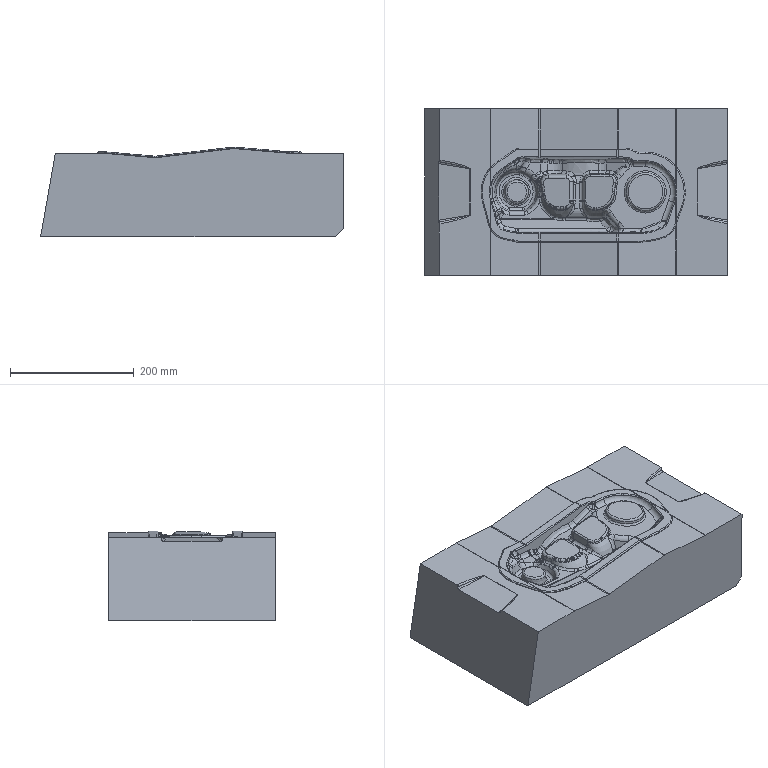NC program | NX | posted with a generic post | part box 490.523 x 270 x 145.452 mm
Lines 1 to 892 of 192747:
N10 G17 G21 G94 G90
(FIXED_CONTOUR , TOOL : 6.)
N12 T00 M6
N14 G54
N16 G17 G0 G90 X-85.619 Y71.107 S3000 M3
N18 G43 Z100. H0
N20 Z5.2
N22 G94 G1 Z0.4 F2500.
N24 X-86.787 Y69.405
N26 X-87.928 Y67.935
N28 Y67.84
N30 X-85.569 Y70.881 Z0.2
N32 Y71.005
N34 X-84.81 Y72.233
N36 X-84.104 Y73.498
N38 X-82.98 Y75.839
N40 X-82.866 Y76.096 Z0.178
N42 X-82.621 Y76.604 Z0.133
N44 X-82.287 Y77.38 Z0.067
N46 X-81.952 Y78.155 Z0.
N48 X-81.954 Y78.15
N50 X-83.083 Y75.364
N52 Y75.2
N54 Z5.2
N56 G0 Z100.
N58 X-19.722 Y93.035
N60 Z1.6
N62 G1 Z-3.456
N64 X-13.17 Y91.559
N66 X-6.598 Y90.205
N68 X-0.002 Y88.972
N70 X-0.001 Y89.016 Z-3.549
N72 X0. Y89.051 Z-3.642
N74 G2 X-18.281 Y92.786 R370.357
N76 G1 Y92.803
N78 Y92.807
N80 X-16.767 Y92.538 Z-3.828
N82 Y92.534
N84 Y92.517
N86 X-15.395 Y92.209
N88 X-7.747 Y90.592
N90 X0. Y89.128
N92 Y89.17 Z-3.921
N94 Y89.198 Z-4.014
N96 X-6.896 Y90.494
N98 X-13.7 Y91.909
N100 X-15.252 Y92.251
N102 Y92.271
N104 X-14.495 Y92.137 Z-4.107
N106 X-14.174 Y92.092 Z-4.138
N108 X-13.99 Y92.047 Z-4.169
N110 X-13.737 Y92.003 Z-4.2
N112 Y91.998
N114 Y91.981
N116 X-12.039 Y91.614
N118 X-6.063 Y90.392
N120 X0. Y89.263
N122 Y89.295 Z-4.293
N124 Y89.316 Z-4.386
N126 X-2.373 Y89.761
N128 X-10.421 Y91.327
N130 X-12.223 Y91.711
N132 Y91.729
N134 Y91.733
N136 X-10.708 Y91.465 Z-4.571
N138 Y91.461
N140 Y91.444
N142 X-8.497 Y90.986
N144 X0. Y89.367
N146 Y89.396 Z-4.664
N148 Y89.412 Z-4.757
N150 X-6.435 Y90.62
N152 X-9.194 Y91.175
N154 Y91.192
N156 Y91.197
N158 X-7.679 Y90.929 Z-4.943
N160 Y90.908
N162 X-4.099 Y90.207
N164 X0. Y89.447
N166 Y89.467 Z-5.036
N168 Y89.477 Z-5.129
N170 X-0.578 Y89.582
N172 X-6.164 Y90.641
N174 Y90.657
N176 Y90.662
N178 X-4.65 Y90.391 Z-5.315
N180 Y90.387
N182 Y90.369
N184 X-0.004 Y89.506
N186 X-0.003 Y89.526 Z-5.501
N188 X-3.135 Y90.103
N190 Y90.12
N192 Y90.124
N194 Z1.6
N196 G0 Z100.
N198 X0.004 Y180.967
N200 Z1.6
N202 G1 Z-3.614
N204 X-8.082 Y179.426
N206 X-16.134 Y177.736
N208 X-18.504 Y177.176
N210 Y177.159
N212 X-16.962 Y177.432 Z-3.804
N214 Y177.449
N216 X-14.338 Y178.042
N218 X-7.468 Y179.472
N220 X-0.573 Y180.773
N222 X0.003 Y180.888
N224 X0.004 Y180.841 Z-3.898
N226 Y180.822 Z-3.993
N228 X-3.565 Y180.152
N230 X-4.164 Y180.056
N232 X-12.543 Y178.358
N234 X-15.42 Y177.72
N236 Y177.704
N238 X-13.878 Y177.978 Z-4.182
N240 Y177.995
N242 X-12.26 Y178.347
N244 X-7.322 Y179.366
N246 X-2.368 Y180.307
N248 X0.004 Y180.748
N250 Y180.71 Z-4.277
N252 Y180.69 Z-4.372
N254 X-8.353 Y179.115
N256 X-12.336 Y178.268
N258 Y178.251
N260 X-10.794 Y178.524 Z-4.561
N262 Y178.541
N264 X-8.56 Y179.001
N266 X0.004 Y180.638
N268 Y180.608 Z-4.656
N270 Y180.591 Z-4.75
N272 X-6.576 Y179.352
N274 X-9.252 Y178.814
N276 Y178.797
N278 X-7.71 Y179.068 Z-4.94
N280 Y179.085
N282 X-6.558 Y179.318
N284 X0.003 Y180.565
N286 X0. Y180.534 Z-5.034
N288 Y180.528 Z-5.129
N290 X-0.573 Y180.43
N292 X-6.168 Y179.358
N294 Y179.341
N296 X-4.626 Y179.617 Z-5.318
N298 Y179.634
N300 X0.003 Y180.501
N302 Y180.475 Z-5.508
N304 X-3.084 Y179.905
N306 Y179.888
N308 Z1.6
N310 G0 Z100.
N312 X-164.272 Y125.065
N314 Z11.2
N316 G1 Z5.572
N318 G2 X-164.29 Y145.109 R32.234
N320 G1 X-163.918 Y146.241 Z5.539
N322 X-163.819 Y146.523 Z5.531
N324 X-163.28 Y147.922 Z5.489
N326 X-162.67 Y149.293 Z5.448
N328 X-162.405 Y149.83 Z5.431
N330 X-161.863 Y150.895 Z5.398
N332 X-161.42 Y151.668 Z5.373
N334 G3 X-161.471 Y118.63 R32.426
N336 G1 X-161.317 Y118.389 Z5.362
N338 X-161.034 Y117.89 Z5.34
N340 X-160.268 Y116.677 Z5.285
N342 X-160.109 Y116.438 Z5.274
N344 X-159.278 Y115.268 Z5.219
N346 X-158.752 Y114.592 Z5.186
N348 X-158.573 Y114.37 Z5.175
N350 X-158.734 Y114.56
N352 X-159.247 Y115.191
N354 X-159.867 Y116.038
N356 G2 X-165.436 Y141.376 R32.467
N358 X-158.607 Y155.835 R32.151
N360 G1 X-158.278 Y156.266 Z5.131
N362 X-157.935 Y156.685 Z5.087
N364 X-157.237 Y157.513 Z4.998
N366 X-157.05 Y157.708 Z4.976
N368 G3 X-165.983 Y138.11 R32.384
N370 G1 X-166.115 Y135.573
N372 X-166.05 Y133.033
N374 X-165.965 Y131.842
N376 X-165.88 Y131.246
N378 X-165.832 Y130.764
N380 X-165.731 Y130.054
N382 X-165.615 Y129.458
N384 X-165.524 Y128.862
N386 G3 X-157.059 Y112.536 R32.534
N388 G1 X-156.677 Y112.126 Z4.948
N390 X-156.098 Y111.515 Z4.906
N392 X-155.489 Y110.933 Z4.863
N394 X-154.877 Y110.356 Z4.82
N396 X-154.243 Y109.808 Z4.778
N398 G2 X-165.831 Y130.354 R32.559
N400 X-165.365 Y142.358 R32.535
N402 X-160.052 Y154.259 R32.552
N404 G1 X-158.428 Y156.335
N406 X-156.639 Y158.271
N408 X-155.462 Y159.386
N410 X-154.231 Y160.442
N412 X-153.779 Y160.824 Z4.745
N414 X-153.553 Y161.016 Z4.728
N416 X-152.384 Y161.924 Z4.646
N418 X-151.419 Y162.605 Z4.579
N420 X-152.824 Y161.638
N422 X-153.259 Y161.294
N424 X-153.616 Y161.042
N426 G3 X-165.08 Y143.76 R32.349
N428 G1 X-165.698 Y141.015
N430 X-166.086 Y138.227
N432 X-166.241 Y135.417
N434 G3 X-159.781 Y115.485 R33.243
N436 G1 X-158.044 Y113.343
N438 X-156.13 Y111.357
N440 X-154.054 Y109.541
N442 X-153.616 Y109.196
N444 X-153.259 Y108.944
N446 X-152.661 Y108.48
N448 X-151.408 Y107.622
N450 X-151.177 Y107.471 Z4.563
N452 X-150.951 Y107.312 Z4.546
N454 X-149.551 Y106.429 Z4.447
N456 X-148.831 Y106.025 Z4.397
N458 X-148.594 Y105.885 Z4.381
N460 G2 X-164.177 Y123.473 R32.567
N462 X-157.009 Y158.119 R33.181
N464 X-148.592 Y164.345 R32.559
N466 G1 X-148.09 Y164.623 Z4.345
N468 X-146.805 Y165.267 Z4.255
N470 X-146.282 Y165.503 Z4.219
N472 X-145.756 Y165.731 Z4.182
N474 G3 X-163.495 Y148.58 R32.442
N476 X-165.617 Y128.266 R33.346
N478 G1 X-165.352 Y127.074
N480 X-165.202 Y126.478
N482 G3 X-153.858 Y109.164 R33.176
N484 G1 X-153.259 Y108.733
N486 X-152.661 Y108.268
N488 X-152.289 Y108.004
N490 G3 X-145.766 Y104.506 R33.729
N492 G1 X-145.51 Y104.404 Z4.164
N494 X-145.258 Y104.291 Z4.146
N496 X-144.489 Y103.987 Z4.092
N498 X-143.715 Y103.695 Z4.038
N500 X-142.93 Y103.442 Z3.984
N502 G2 X-151.418 Y107.34 R31.827
N504 X-160.993 Y116.943 R32.498
N506 X-155.055 Y160.163 R33.378
N508 X-142.948 Y166.794 R32.328
N510 G1 X-142.666 Y166.881 Z3.964
N512 X-142.106 Y167.07 Z3.924
N514 X-140.682 Y167.456 Z3.825
N516 X-140.396 Y167.526 Z3.805
N518 X-140.108 Y167.586 Z3.785
N520 G3 X-155.265 Y160.021 R31.836
N522 X-163.084 Y149.667 R33.015
N524 X-157.427 Y112.312 R33.489
N526 G1 X-155.449 Y110.37
N528 X-153.315 Y108.6
N530 G3 X-140.119 Y102.657 R31.84
N532 G1 X-138.996 Y102.402 Z3.706
N534 X-137.578 Y102.166 Z3.607
N536 X-137.294 Y102.126 Z3.587
N538 X-139.945 Y102.528
N540 G2 X-158.648 Y113.628 R32.465
N542 G1 X-160.302 Y115.768
N544 X-161.774 Y118.038
N546 X-163.053 Y120.422
N548 G2 X-166.231 Y131.321 R33.907
N550 X-153.796 Y161.324 R33.477
N552 X-137.314 Y168.103 R31.937
N554 G1 X-137.032 Y168.151 Z3.567
N556 X-135.9 Y168.288 Z3.488
N558 X-135.616 Y168.316 Z3.468
N560 X-134.481 Y168.387 Z3.388
N562 G3 X-150.082 Y163.93 R31.865
N564 G1 X-152.328 Y162.479
N566 X-154.457 Y160.861
N568 G3 X-164.036 Y122.558 R33.577
N570 X-152.985 Y108.227 R33.222
N572 X-134.481 Y101.859 R32.008
N574 G1 X-134.201 Y101.828 Z3.369
N576 X-133.921 Y101.812 Z3.349
N578 X-132.52 Y101.791 Z3.25
N580 X-131.682 Y101.814 Z3.19
N582 G2 X-149.667 Y106.013 R32.181
N584 X-164.956 Y125.02 R33.356
N586 X-153.743 Y161.482 R33.609
N588 X-137.125 Y168.306 R32.658
N590 G1 X-134.405 Y168.481
N592 X-131.683 Y168.425
N594 X-130.838 Y168.406 Z3.13
N596 X-129.155 Y168.261 Z3.011
N598 X-128.877 Y168.22 Z2.991
N600 X-131.57 Y168.509
N602 G3 X-137.692 Y168.311 R35.795
N604 X-152.062 Y162.767 R32.727
N606 G1 X-154.457 Y160.954
N608 G3 X-159.986 Y115.156 R33.662
N610 G1 X-158.363 Y113.137
N612 G3 X-147.904 Y105.025 R33.306
N614 X-128.879 Y102.017 R32.12
N616 G1 X-128.308 Y102.08 Z2.952
N618 X-127.737 Y102.153 Z2.912
N620 X-127.453 Y102.198 Z2.892
N622 X-126.325 Y102.409 Z2.813
N624 X-126.046 Y102.472 Z2.793
N626 G2 X-148.003 Y105.025 R32.317
N628 G1 X-150.392 Y106.346
N630 G2 X-160.327 Y115.576 R33.664
N632 X-144.147 Y166.838 R33.645
N634 X-126.058 Y167.769 R32.242
N636 G1 X-125.775 Y167.73 Z2.773
N638 X-124.665 Y167.471 Z2.694
N640 X-124.388 Y167.404 Z2.674
N642 X-123.295 Y167.09 Z2.595
N644 G3 X-139.592 Y168.118 R32.546
N646 G1 X-142.053 Y167.537
N648 X-144.462 Y166.768
N650 X-146.805 Y165.817
N652 X-149.068 Y164.689
N654 X-151.488 Y163.233
N656 X-153.778 Y161.58
N658 X-155.921 Y159.74
N660 G3 X-157.017 Y111.58 R33.682
N662 G1 X-156.852 Y111.407
N664 G3 X-139.237 Y102.045 R33.451
N666 X-124.723 Y102.716 R32.48
N668 G1 X-123.284 Y103.155
N670 X-122.997 Y103.225 Z2.575
N672 X-122.713 Y103.308 Z2.555
N674 X-121.317 Y103.788 Z2.456
N676 X-120.493 Y104.108 Z2.396
N678 X-120.928 Y103.931
N680 X-121.118 Y103.833
N682 X-121.527 Y103.692
N684 X-122.697 Y103.237
N686 G2 X-129.31 Y101.709 R37.844
N688 X-134.1 Y101.457 R37.107
N690 G1 X-134.699 Y101.499
N692 G2 X-145.525 Y103.833 R32.829
N694 G1 X-146.075 Y104.08
N696 X-146.673 Y104.329
N698 G2 X-151.438 Y163.304 R33.725
N700 X-139.114 Y168.256 R33.424
N702 X-120.49 Y166.129 R32.461
N704 G1 X-119.714 Y165.829 Z2.342
N706 X-118.202 Y165.138 Z2.234
N708 X-117.711 Y164.883 Z2.198
N710 G3 X-143.895 Y167.038 R32.59
N712 X-155.146 Y160.521 R33.727
N714 G1 X-157.129 Y158.641
N716 X-158.953 Y156.607
N718 X-160.607 Y154.432
N720 X-162.079 Y152.13
N722 G3 X-150.864 Y106.538 R33.734
N724 X-131.312 Y101.464 R33.198
N726 X-117.728 Y105.347 R32.66
N728 G1 X-116.949 Y105.737 Z2.143
N730 X-116.694 Y105.875 Z2.125
N732 X-115.44 Y106.602 Z2.035
N734 X-114.954 Y106.915 Z1.999
N736 G2 X-137.826 Y101.705 R32.613
N738 G1 X-140.427 Y102.184
N740 X-142.983 Y102.868
N742 X-145.476 Y103.752
N744 X-146.075 Y104.022
N746 X-146.673 Y104.262
N748 X-147.045 Y104.429
N750 X-148.469 Y105.127
N752 X-149.068 Y105.448
N754 X-151.464 Y106.881
N756 G2 X-161.247 Y116.7 R33.77
N758 X-147.284 Y165.693 R33.771
N760 X-124.949 Y167.824 R32.947
N762 X-114.962 Y163.331 R32.648
N764 G1 X-114.009 Y162.723 Z1.933
N766 X-112.634 Y161.73 Z1.834
N768 X-112.192 Y161.381 Z1.801
N770 G3 X-136.93 Y168.684 R32.74
N772 X-150.266 Y164.136 R33.753
N774 X-153.137 Y108.024 R33.776
N776 X-131.385 Y101.369 R33.627
N778 G1 X-128.772 Y101.605
N780 G3 X-112.189 Y108.864 R32.871
N782 G1 X-111.518 Y109.387 Z1.755
N784 X-111.088 Y109.756 Z1.724
N786 X-110.237 Y110.505 Z1.663
N788 X-109.421 Y111.287 Z1.602
N790 G2 X-128.439 Y101.606 R33.041
N792 X-145.782 Y103.833 R33.43
N794 X-153.441 Y162.018 R33.798
N796 G1 X-151.108 Y163.642
N798 X-148.646 Y165.064
N800 X-146.075 Y166.274
N802 X-145.782 Y166.405
N804 G2 X-123.666 Y167.597 R33.229
N806 X-109.419 Y158.947 R33.26
N808 G1 X-108.997 Y158.535 Z1.583
N810 X-107.994 Y157.448 Z1.536
N812 X-107.229 Y156.542 Z1.498
N814 X-106.851 Y156.086 Z1.479
N816 X-105.956 Y154.91 Z1.432
N818 X-105.785 Y154.67 Z1.422
N820 X-105.623 Y154.424 Z1.413
N822 X-105.455 Y154.183 Z1.404
N824 G3 X-113.728 Y162.77 R32.793
N826 G1 X-116.018 Y164.278
N828 X-118.423 Y165.595
N830 X-120.928 Y166.711
N832 G3 X-146.075 Y166.303 R33.323
N834 G1 X-148.568 Y165.137
N836 X-150.959 Y163.773
N838 X-153.23 Y162.218
N840 X-155.368 Y160.483
N842 G3 X-157.139 Y111.44 R33.804
N844 X-128.431 Y101.575 R33.872
N846 X-105.482 Y116.019 R32.97
N848 G1 X-105.148 Y116.489 Z1.383
N850 X-104.985 Y116.726 Z1.372
N852 X-104.219 Y117.949 Z1.32
N854 X-104.07 Y118.196 Z1.31
N856 X-103.505 Y119.203 Z1.268
N858 X-103.236 Y119.712 Z1.247
N860 X-102.724 Y120.74 Z1.205
N862 G2 X-121.341 Y103.328 R33.391
N864 G1 X-123.922 Y102.477
N866 G2 X-153.244 Y108.004 R33.808
N868 G1 X-155.438 Y109.786
N870 X-157.476 Y111.744
N872 X-159.343 Y113.866
N874 G2 X-153.816 Y161.789 R33.799
N876 G1 X-153.244 Y162.234
N878 G2 X-126.317 Y168.342 R33.905
N880 X-103.898 Y151.813 R33.206
N882 G1 X-102.783 Y149.621
N884 X-102.706 Y149.454
N886 Z6.605
N888 G0 Z9.005
N890 X-99.98 Y140.994
N892 Z6.605
N894 G1 Z1.007
N896 G3 X-110.734 Y160.55 R34.127
N898 X-133.196 Y169.017 R33.186
N900 X-166.844 Y136.897 R33.962
N902 X-146.727 Y104.155 R33.873
N904 X-125.119 Y102.136 R33.922
N906 G1 X-123.922 Y102.441
N908 G3 X-103.56 Y118.837 R33.366
N910 X-99.963 Y129.342 R34.667
N912 G1 Z6.4
N914 G0 Z100.
N916 X-102.441 Y149.336
N918 Z6.4
N920 G1 Z0.808
N922 G2 X-107.461 Y112.96 R34.453
N924 X-118.524 Y104.429 R33.412
N926 X-147.871 Y104.668 R33.813
N928 X-164.557 Y147.558 R33.857
N930 X-121.377 Y167.003 R34.003
N932 X-104.949 Y153.891 R33.172
N934 G1 X-103.605 Y151.663
N936 X-102.441 Y149.336
N938 X-102.394 Y149.357 Z0.709
N940 X-102.377 Y149.365 Z0.61
N942 G3 X-111.814 Y161.615 R33.797
N944 X-123.628 Y167.76 R33.153
N946 X-165.845 Y143.76 R34.05
N948 X-149.068 Y105.245 R33.907
N950 X-121.875 Y103.028 R34.083
N952 X-108.459 Y111.762 R32.992
N954 X-99.872 Y128.835 R34.
N956 X-101.461 Y147.154 R34.535
N958 G1 X-102.377 Y149.365
N960 Z6.4
N962 G0 Z100.
N964 X-167.07 Y137.895
N966 Z10.
N968 G1 Z0.411
N970 Y136.445
N972 X-166.998 Y137.308
N974 X-166.638 Y140.185
N976 G2 X-128.546 Y168.789 R34.085
N978 X-102.761 Y150.315 R33.363
N980 X-109.732 Y110.388 R34.322
N982 X-129.31 Y101.366 R33.362
N984 G1 X-129.909 Y101.292
N986 X-131.106 Y101.205
N988 X-132.226 Y101.181
N990 G2 X-166.83 Y131.573 R34.059
N992 G1 X-167.028 Y133.406
N994 Z9.561
N996 G0 Z11.961
N998 X-164.662 Y122.521
N1000 Z9.561
N1002 G1 Z0.213
N1004 X-164.635 Y122.476
N1006 X-164.036 Y121.15
N1008 G3 X-118.418 Y104.394 R34.154
N1010 X-104.571 Y116.591 R33.416
N1012 X-107.756 Y157.869 R34.349
N1014 X-123.632 Y167.808 R33.802
N1016 X-164.542 Y147.932 R34.195
N1018 G1 X-164.658 Y147.769
N1020 Z9.363
N1022 G0 Z11.763
N1024 X-162.355 Y152.492
N1026 Z9.363
N1028 G1 Z0.014
N1030 X-161.641 Y153.524
N1032 G2 X-114.564 Y163.724 R34.161
N1034 X-100.352 Y144.37 R33.674
N1036 X-106.376 Y113.963 R34.352
N1038 X-130.508 Y101.213 R33.711
N1040 X-161.788 Y116.943 R34.169
N1042 G1 X-162.361 Y117.747
N1044 Z9.164
N1046 G0 Z11.564
N1048 X-160.026 Y114.272
N1050 Z9.164
N1052 G1 Z-0.184
N1054 X-159.712 Y113.964
N1056 G3 X-128.584 Y101.398 R34.232
N1058 X-100.765 Y124.341 R33.707
N1060 G1 X-100.455 Y125.286
N1062 X-100.295 Y125.882
N1064 G3 X-106.559 Y156.571 R34.301
N1066 X-118.597 Y165.965 R34.067
N1068 X-158.18 Y158.062 R34.283
N1070 G1 X-159.965 Y156.014
N1072 X-160.019 Y155.972
N1074 Z8.966
N1076 G0 Z11.366
N1078 X-157.686 Y158.716
N1080 Z8.966
N1082 G1 Z-0.383
N1084 X-157.403 Y158.929
N1086 G2 X-113.172 Y162.83 R34.263
N1088 X-110.151 Y160.404 R36.808
N1090 X-99.547 Y141.376 R34.02
N1092 G1 X-99.463 Y140.78
N1094 X-99.374 Y140.353
N1096 G2 X-101.276 Y122.776 R34.557
N1098 X-112.227 Y108.116 R33.746
N1100 X-132.304 Y101.1 R33.979
N1102 X-156.45 Y110.388 R34.253
N1104 G1 X-157.599 Y111.468
N1106 X-157.682 Y111.518
N1108 Z8.767
N1110 G0 Z11.167
N1112 X-155.345 Y109.27
N1114 Z8.767
N1116 G1 Z-0.581
N1118 X-155.195 Y109.196
N1120 X-154.444 Y108.6
N1122 G3 X-110.151 Y109.807 R34.285
N1124 X-110.151 Y160.431 R34.166
N1126 X-152.862 Y162.83 R34.281
N1128 G1 X-153.259 Y162.55
N1130 X-155.303 Y160.993
N1132 Z8.569
N1134 G0 Z10.969
N1136 X-153.016 Y162.841
N1138 Z8.569
N1140 G1 Z-0.78
N1142 X-152.661 Y163.02
N1144 G2 X-108.763 Y159.131 R34.334
N1146 X-108.648 Y111.224 R34.171
N1148 X-152.661 Y107.219 R34.331
N1150 G1 X-153.002 Y107.392
N1152 Z8.37
N1154 G0 Z10.77
N1156 X-150.644 Y105.816
N1158 Z8.37
N1160 G1 Z-0.978
N1162 X-150.492 Y105.783
N1164 X-149.154 Y105.069
N1166 G3 X-106.559 Y113.542 R34.248
N1168 X-102.545 Y150.515 R34.174
N1170 X-132.304 Y169.189 R34.082
N1172 X-150.492 Y164.455 R34.789
N1174 G1 X-150.652 Y164.421
N1176 Z8.172
N1178 G0 Z10.572
N1180 X-148.255 Y165.711
N1182 Z8.172
N1184 G1 Z-1.177
N1186 X-148.246 Y165.704
N1188 G2 X-119.03 Y166.232 R34.614
N1190 X-99.13 Y139.416 R34.083
N1192 X-104.88 Y115.751 R34.218
N1194 X-144.877 Y103.123 R34.302
N1196 G1 X-146.537 Y103.773
N1198 X-148.163 Y104.502
N1200 X-148.191 Y104.484
N1202 Z9.173
N1204 G0 Z10.373
N1206 X-145.959 Y103.435
N1208 Z7.973
N1210 G1 Z-1.375
N1212 X-145.787 Y103.43
N1214 G3 X-109.522 Y110.341 R34.448
N1216 X-125.718 Y168.437 R34.091
N1218 X-145.793 Y166.808 R34.709
N1220 G1 X-145.957 Y166.803
N1222 X-145.491 Y166.928 Z-1.4
N1224 X-144.699 Y167.234 Z-1.45
N1226 X-144.386 Y167.353 Z-1.475
N1228 X-144.192 Y167.421 Z-1.499
N1230 X-143.871 Y167.548 Z-1.524
N1232 X-143.718 Y167.604 Z-1.549
N1234 X-143.607 Y167.677 Z-1.574
N1236 X-143.081 Y167.779
N1238 G2 X-104.548 Y154.005 R34.379
N1240 X-118.533 Y104.214 R34.09
N1242 G1 X-119.731 Y103.678
N1244 X-120.329 Y103.443
N1246 G2 X-143.081 Y102.459 R34.458
N1248 G1 X-143.624 Y102.567
N1250 Z8.776
N1252 G0 Z9.976
N1254 X-141.234 Y101.861
N1256 Z7.576
N1258 G1 Z-1.772
N1260 X-141.103 Y101.897
N1262 G3 X-107.961 Y111.894 R34.471
N1264 X-120.589 Y166.907 R34.101
N1266 X-141.101 Y168.342 R34.56
N1268 G1 X-141.233 Y168.377
N1270 X-140.939 Y168.44 Z-1.797
N1272 X-140.65 Y168.493 Z-1.822
N1274 X-140.053 Y168.633 Z-1.872
N1276 X-139.176 Y168.807 Z-1.946
N1278 X-138.893 Y168.858 Z-1.971
N1280 X-138.89 Y168.853
N1282 X-136.932 Y169.074
N1284 G2 X-99.404 Y141.351 R34.264
N1286 X-125.943 Y101.712 R34.156
N1288 X-138.291 Y101.329 R34.875
N1290 G1 X-138.89 Y101.385
N1292 X-138.903 Y101.373
N1294 Z8.379
N1296 G0 Z9.579
N1298 X-136.417 Y101.01
N1300 Z8.379
N1302 G1 Z-2.169
N1304 X-135.896 Y101.028
N1306 G3 X-112.455 Y107.83 R34.533
N1308 X-99.402 Y141.376 R34.213
N1310 X-134.699 Y169.272 R34.301
N1312 G1 X-136.495 Y169.185
N1314 X-136.555 Y169.209
N1316 X-135.393 Y169.298 Z-2.269
N1318 X-134.807 Y169.362 Z-2.318
N1320 X-134.23 Y169.376 Z-2.368
N1322 X-134.1 Y169.345
N1324 G2 X-121.777 Y167.397 R36.486
N1326 X-100.466 Y124.682 R34.202
N1328 X-132.304 Y100.929 R34.288
N1330 G1 X-134.1 Y100.893
N1332 X-134.23 Y100.862
N1334 X-133.637 Y100.858 Z-2.417
N1336 X-133.332 Y100.837 Z-2.442
N1338 X-132.45 Y100.851 Z-2.517
N1340 X-131.859 Y100.85 Z-2.566
N1342 X-131.804 Y100.896
N1344 G3 X-116.708 Y105.079 R35.151
N1346 X-108.006 Y158.417 R34.177
N1348 G1 X-110.049 Y160.434
N1350 G3 X-127.023 Y168.787 R34.428
N1352 G1 X-129.399 Y169.144
N1354 X-131.793 Y169.341
N1356 X-131.853 Y169.387
N1358 X-131.551 Y169.377 Z-2.591
N1360 X-130.925 Y169.384 Z-2.641
N1362 X-130.657 Y169.331 Z-2.665
N1364 X-130.071 Y169.287 Z-2.715
N1366 X-129.759 Y169.288 Z-2.74
N1368 X-129.493 Y169.234 Z-2.765
N1370 X-129.425 Y169.177
N1372 G2 X-113.001 Y162.83 R34.92
N1374 X-120.67 Y103.237 R34.186
N1376 G1 X-122.803 Y102.487
N1378 X-124.978 Y101.873
N1380 X-127.188 Y101.397
N1382 X-129.423 Y101.062
N1384 X-129.5 Y100.999
N1386 X-129.203 Y101.014 Z-2.787
N1388 X-128.959 Y101.069 Z-2.809
N1390 X-128.154 Y101.184 Z-2.875
N1392 X-127.895 Y101.227 Z-2.897
N1394 X-127.285 Y101.282 Z-2.941
N1396 X-127.125 Y101.355 Z-2.963
N1398 X-127.12 Y101.373
N1400 G3 X-114.885 Y106.124 R36.128
N1402 X-117.386 Y165.526 R34.201
N1404 G1 X-119.721 Y166.626
N1406 X-122.13 Y167.552
N1408 X-124.601 Y168.3
N1410 X-127.119 Y168.864
N1412 X-127.126 Y168.889
N1414 X-126.715 Y168.869 Z-2.988
N1416 X-126.528 Y168.78 Z-3.013
N1418 X-126.236 Y168.723 Z-3.038
N1420 X-125.931 Y168.673 Z-3.062
N1422 X-125.647 Y168.613 Z-3.087
N1424 X-125.339 Y168.566 Z-3.112
N1426 X-124.804 Y168.427 Z-3.162
N1428 X-124.766 Y168.366
N1430 G2 X-110.765 Y161.087 R35.121
N1432 X-102.236 Y150.009 R34.209
N1434 X-117.934 Y104.423 R34.209
N1436 G1 X-120.152 Y103.419
N1438 X-122.433 Y102.568
N1440 X-124.766 Y101.872
N1442 X-124.783 Y101.826
N1444 X-124.461 Y101.88 Z-3.184
N1446 X-124.252 Y101.975 Z-3.206
N1448 X-123.725 Y102.126 Z-3.25
N1450 X-123.373 Y102.173 Z-3.272
N1452 X-123.193 Y102.275 Z-3.294
N1454 X-122.939 Y102.354 Z-3.316
N1456 X-122.66 Y102.425 Z-3.338
N1458 X-122.442 Y102.514 Z-3.36
N1460 X-122.438 Y102.525
N1462 X-120.772 Y103.15
N1464 X-119.132 Y103.842
N1466 G3 X-115.189 Y164.311 R34.233
N1468 G1 X-117.519 Y165.623
N1470 X-119.94 Y166.759
N1472 X-122.438 Y167.712
N1474 X-122.443 Y167.73
N1476 X-122.116 Y167.662 Z-3.382
N1478 X-121.912 Y167.556 Z-3.404
N1480 X-121.393 Y167.38 Z-3.448
N1482 X-121.12 Y167.298 Z-3.47
N1484 X-120.884 Y167.199 Z-3.493
N1486 X-120.378 Y167.016 Z-3.537
N1488 X-120.131 Y166.92 Z-3.559
N1490 X-120.104 Y166.874
N1492 X-118.074 Y165.908
N1494 X-115.604 Y164.577
N1496 X-113.251 Y163.048
N1498 X-111.031 Y161.332
N1500 X-108.959 Y159.44
N1502 X-107.049 Y157.385
N1504 G2 X-110.459 Y109.409 R34.239
N1506 X-119.132 Y103.825 R34.242
N1508 G1 X-120.047 Y103.404
N1510 X-120.099 Y103.372
N1512 X-120.124 Y103.32
N1514 X-119.832 Y103.423 Z-3.581
N1516 X-119.326 Y103.668 Z-3.625
N1518 X-118.282 Y104.143 Z-3.713
N1520 X-117.766 Y104.384 Z-3.757
N1522 X-117.727 Y104.455
N1524 X-115.415 Y105.769
N1526 X-114.342 Y106.435
N1528 X-112.096 Y108.036
N1530 X-109.985 Y109.813
N1532 X-108.025 Y111.754
N1534 G3 X-112.952 Y162.834 R34.264
N1536 G1 X-115.283 Y164.401
N1538 X-117.727 Y165.783
N1540 X-117.768 Y165.855
N1542 X-117.507 Y165.714 Z-3.779
N1544 X-116.938 Y165.454 Z-3.823
N1546 X-116.716 Y165.294 Z-3.845
N1548 X-116.449 Y165.155 Z-3.867
N1550 X-115.941 Y164.867 Z-3.912
N1552 X-115.666 Y164.73 Z-3.934
N1554 X-115.424 Y164.583 Z-3.956
N1556 X-115.403 Y164.511
N1558 G2 X-102.999 Y151.51 R35.1
N1560 X-110.75 Y109.138 R34.262
N1562 G1 X-113.012 Y107.344
N1564 X-115.403 Y105.727
N1566 X-115.452 Y105.638
N1568 X-115.198 Y105.782 Z-3.976
N1570 X-114.729 Y106.092 Z-4.015
N1572 X-114.472 Y106.236 Z-4.035
N1574 X-114.241 Y106.392 Z-4.055
N1576 X-113.999 Y106.543 Z-4.075
N1578 X-113.778 Y106.706 Z-4.095
N1580 X-113.528 Y106.852 Z-4.114
N1582 X-113.306 Y107.014 Z-4.134
N1584 X-113.096 Y107.182 Z-4.154
N1586 X-113.077 Y107.216
N1588 X-111.416 Y108.573
N1590 X-109.33 Y110.422
N1592 X-107.402 Y112.435
N1594 G3 X-109.775 Y160.232 R34.27
N1596 G1 X-111.39 Y161.657
N1598 X-113.074 Y162.999
N1600 X-113.088 Y163.052
N1602 X-112.871 Y162.884 Z-4.172
N1604 X-112.635 Y162.721 Z-4.19
N1606 X-112.43 Y162.55 Z-4.208
N1608 X-112.21 Y162.382 Z-4.226
N1610 X-112.004 Y162.211 Z-4.244
N1612 X-111.783 Y162.044 Z-4.262
N1614 X-111.356 Y161.706 Z-4.299
N1616 X-111.156 Y161.533 Z-4.317
N1618 X-110.946 Y161.363 Z-4.335
N1620 X-110.721 Y161.197 Z-4.353
N1622 X-110.699 Y161.114
N1624 G2 X-99.576 Y142.275 R34.813
N1626 X-110.151 Y109.631 R34.372
N1628 G1 X-110.699 Y109.124
N1630 X-110.742 Y109.025
N1632 X-110.527 Y109.223 Z-4.371
N1634 X-110.288 Y109.412 Z-4.389
N1636 X-110.103 Y109.624 Z-4.407
N1638 X-109.426 Y110.207 Z-4.461
N1640 X-109.236 Y110.416 Z-4.479
N1642 X-108.405 Y111.225 Z-4.551
N1644 X-108.355 Y111.34
N1646 G3 X-101.553 Y121.708 R35.978
N1648 X-105.667 Y155.679 R34.296
N1650 G1 X-106.973 Y157.321
N1652 X-108.355 Y158.898
N1654 X-108.421 Y159.026
N1656 X-108.022 Y158.607 Z-4.582
N1658 X-107.842 Y158.388 Z-4.597
N1660 X-107.458 Y157.961 Z-4.628
N1662 X-107.283 Y157.741 Z-4.643
N1664 X-107.054 Y157.54 Z-4.658
N1666 X-106.916 Y157.308 Z-4.673
N1668 X-106.725 Y157.094 Z-4.689
N1670 X-106.521 Y156.883 Z-4.704
N1672 X-106.37 Y156.658 Z-4.719
N1674 X-106.2 Y156.439 Z-4.734
N1676 X-105.988 Y156.226 Z-4.75
N1678 X-105.96 Y156.104
N1680 G2 X-99.267 Y129.619 R34.515
N1682 X-105.96 Y114.134 R34.645
N1684 G1 X-106.033 Y113.964
N1686 Y113.949
N1688 X-105.872 Y114.192 Z-4.764
N1690 X-105.701 Y114.434 Z-4.778
N1692 X-105.348 Y114.918 Z-4.806
N1694 X-105.137 Y115.155 Z-4.821
N1696 X-105.011 Y115.403 Z-4.835
N1698 X-104.78 Y115.632 Z-4.849
N1700 X-104.667 Y115.885 Z-4.863
N1702 X-104.502 Y116.128 Z-4.877
N1704 X-104.024 Y116.863 Z-4.92
N1706 X-103.861 Y117.107 Z-4.934
N1708 X-103.688 Y117.348 Z-4.948
N1710 X-103.613 Y117.539
N1712 X-102.589 Y119.478
N1714 X-101.665 Y121.466
N1716 X-100.843 Y123.499
N1718 G3 X-103.565 Y152.585 R34.568
N1720 G1 X-103.604 Y152.759
N1722 X-103.504 Y152.484 Z-4.96
N1724 X-103.291 Y152.234 Z-4.971
N1726 X-103.208 Y151.955 Z-4.983
N1728 X-102.769 Y151.161 Z-5.018
N1730 X-102.585 Y150.903 Z-5.03
N1732 X-102.5 Y150.626 Z-5.042
N1734 X-102.097 Y149.824 Z-5.077
N1736 X-101.477 Y148.478 Z-5.135
N1738 X-101.323 Y148.214 Z-5.147
N1740 X-101.274 Y147.932
N1742 G2 X-101.274 Y122.307 R34.718
N1744 G1 X-101.3 Y122.083
N1746 Z5.203
N1748 G0 Z6.403
N1750 X-99.015 Y130.805
N1752 Z5.203
N1754 G1 Z-5.345
N1756 X-98.941 Y131.842
N1758 X-98.804 Y134.82
N1760 X-98.904 Y137.801
N1762 X-99.041 Y139.652
N1764 Z5.2
N1766 G0 Z100.
N1768 X-179.768 Y159.19
N1770 Z11.2
N1772 G1 Z6.357
N1774 G2 X-178.476 Y149.023 R12.415
N1776 G1 X-179.155 Y146.723
N1778 Z11.2
N1780 G0 Z100.
N1782 X-180.726 Y132.285